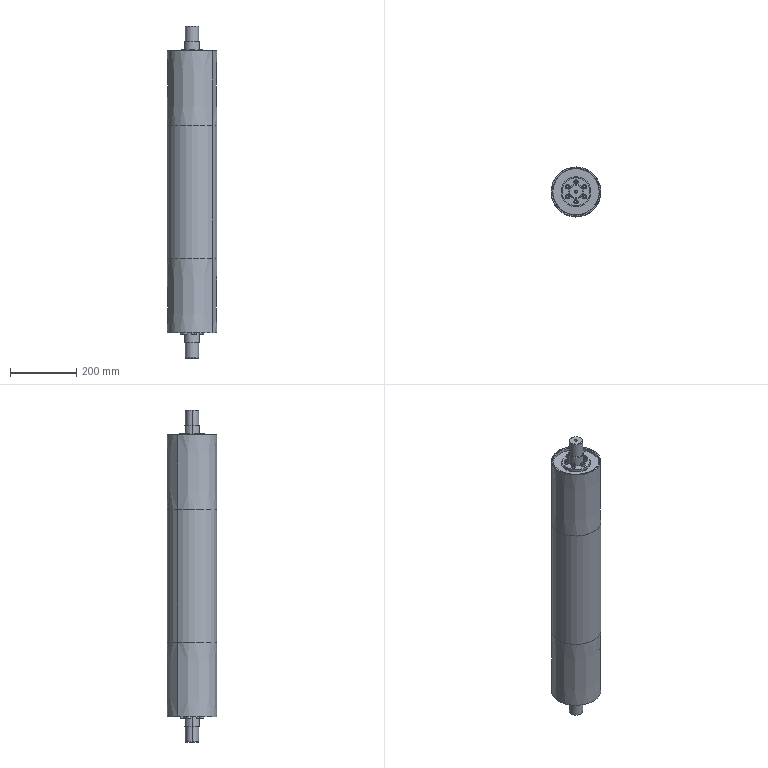Part | SolidWorks | 20 solids | 388 faces | box 150 x 150 x 1000 mm | volume 4622991 mm3 | plane 142 | cylinder 138 | cone 56 | torus 52 | commonest cylinder face diameters 6.647 x44 8 x24 13 x24 75 x8 140 x8 45 x6